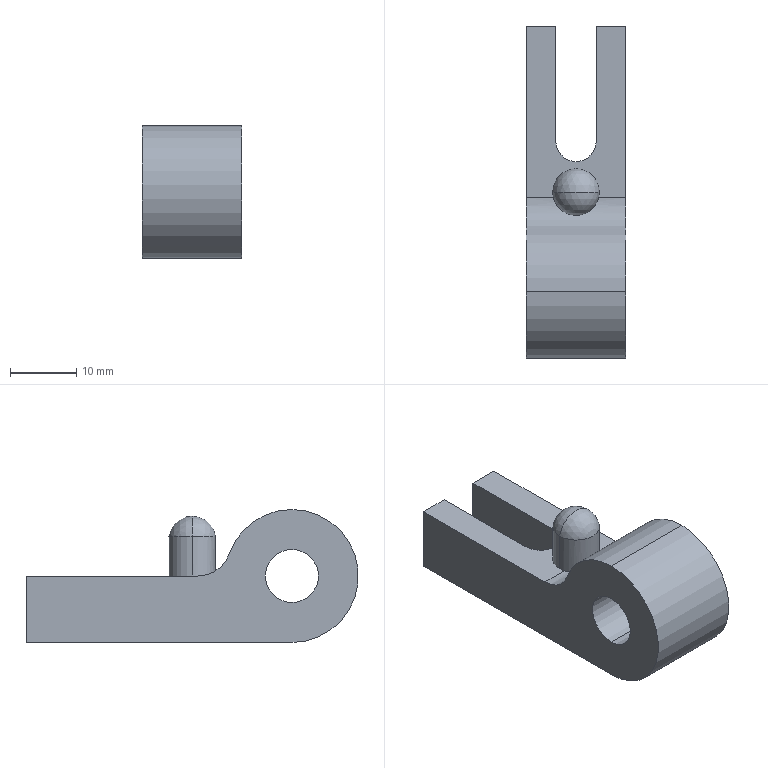Part | SolidWorks | features ICE 4, Fillet 2, Dome 1, Extrusion 1 | 1 solid | 18 faces | box 15 x 50 x 20 mm | volume 7920 mm3 | cylinder 8 | plane 8 | sphere 2 | commonest cylinder face diameters 7 x2 8 x2 20 x2 6.1 x1 10 x1
STEP:
#1=CARTESIAN_POINT('',(3.5,25.,6.));
#2=VERTEX_POINT('',#1);
#3=CARTESIAN_POINT('',(-3.5,25.,6.));
#4=VERTEX_POINT('',#3);
#5=CARTESIAN_POINT('',(0.,25.,6.));
#6=DIRECTION('',(0.,0.,1.));
#7=DIRECTION('',(1.,0.,0.));
#8=AXIS2_PLACEMENT_3D('',#5,#6,#7);
#9=CIRCLE('',#8,3.5);
#10=EDGE_CURVE('',#2,#4,#9,.T.);
#11=ORIENTED_EDGE('',*,*,#10,.T.);
#12=CARTESIAN_POINT('',(0.,25.,9.));
#13=VERTEX_POINT('',#12);
#14=CARTESIAN_POINT('',(0.,25.,5.458));
#15=DIRECTION('',(0.,1.,0.));
#16=DIRECTION('',(-1.,0.,0.));
#17=AXIS2_PLACEMENT_3D('',#14,#15,#16);
#18=CIRCLE('',#17,3.542);
#19=EDGE_CURVE('',#4,#13,#18,.T.);
#20=ORIENTED_EDGE('',*,*,#19,.T.);
#21=CARTESIAN_POINT('',(0.,25.,5.458));
#22=DIRECTION('',(0.,-1.,0.));
#23=DIRECTION('',(0.,0.,-1.));
#24=AXIS2_PLACEMENT_3D('',#21,#22,#23);
#25=CIRCLE('',#24,3.542);
#26=EDGE_CURVE('',#2,#13,#25,.T.);
#27=ORIENTED_EDGE('',*,*,#26,.F.);
#28=EDGE_LOOP('',(#11,#20,#27));
#29=FACE_OUTER_BOUND('',#28,.T.);
#30=CARTESIAN_POINT('',(0.,25.,5.458));
#31=DIRECTION('',(0.,1.,0.));
#32=DIRECTION('',(1.,0.,0.));
#33=AXIS2_PLACEMENT_3D('',#30,#31,#32);
#34=SPHERICAL_SURFACE('',#33,3.542);
#35=ADVANCED_FACE('',(#29),#34,.T.);
#36=ORIENTED_EDGE('',*,*,#10,.F.);
#37=CARTESIAN_POINT('',(3.5,25.,0.));
#38=VERTEX_POINT('',#37);
#39=CARTESIAN_POINT('',(3.5,25.,6.));
#40=DIRECTION('',(0.,0.,-1.));
#41=VECTOR('',#40,1000.);
#42=LINE('',#39,#41);
#43=EDGE_CURVE('',#2,#38,#42,.T.);
#44=ORIENTED_EDGE('',*,*,#43,.T.);
#45=CARTESIAN_POINT('',(-3.5,25.,0.));
#46=VERTEX_POINT('',#45);
#47=CARTESIAN_POINT('',(0.,25.,0.));
#48=DIRECTION('',(0.,0.,1.));
#49=DIRECTION('',(1.,0.,0.));
#50=AXIS2_PLACEMENT_3D('',#47,#48,#49);
#51=CIRCLE('',#50,3.5);
#52=EDGE_CURVE('',#38,#46,#51,.T.);
#53=ORIENTED_EDGE('',*,*,#52,.T.);
#54=CARTESIAN_POINT('',(-3.5,25.,6.));
#55=DIRECTION('',(0.,0.,-1.));
#56=VECTOR('',#55,1000.);
#57=LINE('',#54,#56);
#58=EDGE_CURVE('',#4,#46,#57,.T.);
#59=ORIENTED_EDGE('',*,*,#58,.F.);
#60=EDGE_LOOP('',(#36,#44,#53,#59));
#61=FACE_OUTER_BOUND('',#60,.T.);
#62=CARTESIAN_POINT('',(0.,25.,6.));
#63=DIRECTION('',(0.,0.,-1.));
#64=DIRECTION('',(-1.,0.,0.));
#65=AXIS2_PLACEMENT_3D('',#62,#63,#64);
#66=CYLINDRICAL_SURFACE('',#65,3.5);
#67=ADVANCED_FACE('',(#61),#66,.T.);
#68=CARTESIAN_POINT('',(7.5,10.,-4.));
#69=VERTEX_POINT('',#68);
#70=CARTESIAN_POINT('',(7.5,10.,4.));
#71=VERTEX_POINT('',#70);
#72=CARTESIAN_POINT('',(7.5,10.,0.));
#73=DIRECTION('',(-1.,0.,0.));
#74=DIRECTION('',(0.,0.,1.));
#75=AXIS2_PLACEMENT_3D('',#72,#73,#74);
#76=CIRCLE('',#75,4.);
#77=EDGE_CURVE('',#69,#71,#76,.T.);
#78=ORIENTED_EDGE('',*,*,#77,.F.);
#79=CARTESIAN_POINT('',(-7.5,10.,-4.));
#80=VERTEX_POINT('',#79);
#81=CARTESIAN_POINT('',(7.5,10.,-4.));
#82=DIRECTION('',(-1.,0.,0.));
#83=VECTOR('',#82,1000.);
#84=LINE('',#81,#83);
#85=EDGE_CURVE('',#69,#80,#84,.T.);
#86=ORIENTED_EDGE('',*,*,#85,.T.);
#87=CARTESIAN_POINT('',(-7.5,10.,4.));
#88=VERTEX_POINT('',#87);
#89=CARTESIAN_POINT('',(-7.5,10.,0.));
#90=DIRECTION('',(-1.,0.,0.));
#91=DIRECTION('',(0.,0.,1.));
#92=AXIS2_PLACEMENT_3D('',#89,#90,#91);
#93=CIRCLE('',#92,4.);
#94=EDGE_CURVE('',#80,#88,#93,.T.);
#95=ORIENTED_EDGE('',*,*,#94,.T.);
#96=CARTESIAN_POINT('',(7.5,10.,4.));
#97=DIRECTION('',(-1.,0.,0.));
#98=VECTOR('',#97,1000.);
#99=LINE('',#96,#98);
#100=EDGE_CURVE('',#71,#88,#99,.T.);
#101=ORIENTED_EDGE('',*,*,#100,.F.);
#102=EDGE_LOOP('',(#78,#86,#95,#101));
#103=FACE_OUTER_BOUND('',#102,.T.);
#104=CARTESIAN_POINT('',(7.5,10.,0.));
#105=DIRECTION('',(-1.,0.,0.));
#106=DIRECTION('',(0.,0.,1.));
#107=AXIS2_PLACEMENT_3D('',#104,#105,#106);
#108=CYLINDRICAL_SURFACE('',#107,4.);
#109=ADVANCED_FACE('',(#103),#108,.F.);
#110=CARTESIAN_POINT('',(7.5,10.,10.));
#111=VERTEX_POINT('',#110);
#112=CARTESIAN_POINT('',(7.5,10.,-10.));
#113=VERTEX_POINT('',#112);
#114=CARTESIAN_POINT('',(7.5,10.,0.));
#115=DIRECTION('',(1.,0.,0.));
#116=DIRECTION('',(0.,0.,1.));
#117=AXIS2_PLACEMENT_3D('',#114,#115,#116);
#118=CIRCLE('',#117,10.);
#119=EDGE_CURVE('',#111,#113,#118,.T.);
#120=ORIENTED_EDGE('',*,*,#119,.F.);
#121=CARTESIAN_POINT('',(-7.5,10.,10.));
#122=VERTEX_POINT('',#121);
#123=CARTESIAN_POINT('',(7.5,10.,10.));
#124=DIRECTION('',(-1.,0.,0.));
#125=VECTOR('',#124,1000.);
#126=LINE('',#123,#125);
#127=EDGE_CURVE('',#111,#122,#126,.T.);
#128=ORIENTED_EDGE('',*,*,#127,.T.);
#129=CARTESIAN_POINT('',(-7.5,10.,-10.));
#130=VERTEX_POINT('',#129);
#131=CARTESIAN_POINT('',(-7.5,10.,0.));
#132=DIRECTION('',(-1.,0.,0.));
#133=DIRECTION('',(0.,0.,-1.));
#134=AXIS2_PLACEMENT_3D('',#131,#132,#133);
#135=CIRCLE('',#134,10.);
#136=EDGE_CURVE('',#130,#122,#135,.T.);
#137=ORIENTED_EDGE('',*,*,#136,.F.);
#138=CARTESIAN_POINT('',(7.5,10.,-10.));
#139=DIRECTION('',(-1.,0.,0.));
#140=VECTOR('',#139,1000.);
#141=LINE('',#138,#140);
#142=EDGE_CURVE('',#113,#130,#141,.T.);
#143=ORIENTED_EDGE('',*,*,#142,.F.);
#144=EDGE_LOOP('',(#120,#128,#137,#143));
#145=FACE_OUTER_BOUND('',#144,.T.);
#146=CARTESIAN_POINT('',(7.5,10.,0.));
#147=DIRECTION('',(-1.,0.,0.));
#148=DIRECTION('',(0.,0.,1.));
#149=AXIS2_PLACEMENT_3D('',#146,#147,#148);
#150=CYLINDRICAL_SURFACE('',#149,10.);
#151=ADVANCED_FACE('',(#145),#150,.T.);
#152=CARTESIAN_POINT('',(-3.05,50.,0.));
#153=VERTEX_POINT('',#152);
#154=CARTESIAN_POINT('',(-7.5,50.,0.));
#155=VERTEX_POINT('',#154);
#156=CARTESIAN_POINT('',(7.5,50.,0.));
#157=DIRECTION('',(-1.,0.,0.));
#158=VECTOR('',#157,1000.);
#159=LINE('',#156,#158);
#160=EDGE_CURVE('',#153,#155,#159,.T.);
#161=ORIENTED_EDGE('',*,*,#160,.F.);
#162=CARTESIAN_POINT('',(-3.05,50.,-10.));
#163=VERTEX_POINT('',#162);
#164=CARTESIAN_POINT('',(-3.05,50.,10.));
#165=DIRECTION('',(0.,0.,-1.));
#166=VECTOR('',#165,1000.);
#167=LINE('',#164,#166);
#168=EDGE_CURVE('',#153,#163,#167,.T.);
#169=ORIENTED_EDGE('',*,*,#168,.T.);
#170=CARTESIAN_POINT('',(-7.5,50.,-10.));
#171=VERTEX_POINT('',#170);
#172=CARTESIAN_POINT('',(-7.5,50.,-10.));
#173=DIRECTION('',(-1.,0.,0.));
#174=VECTOR('',#173,1000.);
#175=LINE('',#172,#174);
#176=EDGE_CURVE('',#163,#171,#175,.T.);
#177=ORIENTED_EDGE('',*,*,#176,.T.);
#178=CARTESIAN_POINT('',(-7.5,50.,10.));
#179=DIRECTION('',(0.,0.,1.));
#180=VECTOR('',#179,1000.);
#181=LINE('',#178,#180);
#182=EDGE_CURVE('',#171,#155,#181,.T.);
#183=ORIENTED_EDGE('',*,*,#182,.T.);
#184=EDGE_LOOP('',(#161,#169,#177,#183));
#185=FACE_OUTER_BOUND('',#184,.T.);
#186=CARTESIAN_POINT('',(0.,50.,0.));
#187=DIRECTION('',(0.,-1.,0.));
#188=DIRECTION('',(0.,0.,-1.));
#189=AXIS2_PLACEMENT_3D('',#186,#187,#188);
#190=PLANE('',#189);
#191=ADVANCED_FACE('',(#185),#190,.F.);
#192=CARTESIAN_POINT('',(-3.393,24.142,0.));
#193=VERTEX_POINT('',#192);
#194=CARTESIAN_POINT('',(3.393,24.142,0.));
#195=VERTEX_POINT('',#194);
#196=CARTESIAN_POINT('',(-3.393,24.142,0.));
#197=CARTESIAN_POINT('',(-3.345,23.95,0.));
#198=CARTESIAN_POINT('',(-3.281,23.766,0.011));
#199=CARTESIAN_POINT('',(-3.124,23.411,0.05057));
#200=CARTESIAN_POINT('',(-3.031,23.239,0.0794));
#201=CARTESIAN_POINT('',(-2.818,22.915,0.1501));
#202=CARTESIAN_POINT('',(-2.7,22.765,0.1913));
#203=CARTESIAN_POINT('',(-2.441,22.485,0.2804));
#204=CARTESIAN_POINT('',(-2.3,22.355,0.3287));
#205=CARTESIAN_POINT('',(-1.999,22.121,0.4251));
#206=CARTESIAN_POINT('',(-1.841,22.017,0.4729));
#207=CARTESIAN_POINT('',(-1.507,21.835,0.5628));
#208=CARTESIAN_POINT('',(-1.33,21.757,0.6051));
#209=CARTESIAN_POINT('',(-0.9648,21.63,0.6763));
#210=CARTESIAN_POINT('',(-0.7783,21.582,0.7049));
#211=CARTESIAN_POINT('',(-0.3972,21.517,0.7443));
#212=CARTESIAN_POINT('',(-0.2008,21.5,0.755));
#213=CARTESIAN_POINT('',(0.1939,21.5,0.7552));
#214=CARTESIAN_POINT('',(0.3883,21.516,0.7449));
#215=CARTESIAN_POINT('',(0.7717,21.581,0.7058));
#216=CARTESIAN_POINT('',(0.9624,21.629,0.6767));
#217=CARTESIAN_POINT('',(1.328,21.756,0.6055));
#218=CARTESIAN_POINT('',(1.503,21.833,0.5638));
#219=CARTESIAN_POINT('',(1.839,22.016,0.4735));
#220=CARTESIAN_POINT('',(2.,22.121,0.4247));
#221=CARTESIAN_POINT('',(2.3,22.355,0.3287));
#222=CARTESIAN_POINT('',(2.439,22.483,0.2811));
#223=CARTESIAN_POINT('',(2.699,22.763,0.1916));
#224=CARTESIAN_POINT('',(2.819,22.917,0.1497));
#225=CARTESIAN_POINT('',(3.03,23.238,0.07977));
#226=CARTESIAN_POINT('',(3.122,23.406,0.05121));
#227=CARTESIAN_POINT('',(3.279,23.762,0.01128));
#228=CARTESIAN_POINT('',(3.345,23.95,0.));
#229=CARTESIAN_POINT('',(3.393,24.142,0.));
#230=B_SPLINE_CURVE_WITH_KNOTS('',3,(#196,#197,#198,#199,#200,#201,#202,#203,#204,#205,#206,#207,#208,#209,#210,#211,#212,#213,#214,#215,#216,#217,#218,#219,#220,#221,#222,#223,#224,#225,#226,#227,#228,#229),.UNSPECIFIED.,.F.,.F.,(4,2,2,2,2,2,2,2,2,2,2,2,2,2,2,2,4),(0.,0.0005847,0.001169,0.001754,0.002339,0.002924,0.003508,0.004093,0.004678,0.005262,0.005847,0.006432,0.007017,0.007601,0.008186,0.008771,0.009355),.UNSPECIFIED.);
#231=EDGE_CURVE('',#193,#195,#230,.T.);
#232=ORIENTED_EDGE('',*,*,#231,.F.);
#233=CARTESIAN_POINT('',(-7.5,24.142,0.));
#234=VERTEX_POINT('',#233);
#235=CARTESIAN_POINT('',(7.5,24.142,0.));
#236=DIRECTION('',(1.,0.,0.));
#237=VECTOR('',#236,1000.);
#238=LINE('',#235,#237);
#239=EDGE_CURVE('',#234,#193,#238,.T.);
#240=ORIENTED_EDGE('',*,*,#239,.F.);
#241=CARTESIAN_POINT('',(-7.5,19.428,3.333));
#242=VERTEX_POINT('',#241);
#243=CARTESIAN_POINT('',(-7.5,24.142,5.));
#244=DIRECTION('',(1.,0.,0.));
#245=DIRECTION('',(0.,0.,-1.));
#246=AXIS2_PLACEMENT_3D('',#243,#244,#245);
#247=CIRCLE('',#246,5.);
#248=EDGE_CURVE('',#242,#234,#247,.T.);
#249=ORIENTED_EDGE('',*,*,#248,.F.);
#250=CARTESIAN_POINT('',(7.5,19.428,3.333));
#251=VERTEX_POINT('',#250);
#252=CARTESIAN_POINT('',(7.5,19.428,3.333));
#253=DIRECTION('',(-1.,0.,0.));
#254=VECTOR('',#253,1000.);
#255=LINE('',#252,#254);
#256=EDGE_CURVE('',#251,#242,#255,.T.);
#257=ORIENTED_EDGE('',*,*,#256,.F.);
#258=CARTESIAN_POINT('',(7.5,24.142,0.));
#259=VERTEX_POINT('',#258);
#260=CARTESIAN_POINT('',(7.5,24.142,5.));
#261=DIRECTION('',(-1.,0.,0.));
#262=DIRECTION('',(0.,0.,1.));
#263=AXIS2_PLACEMENT_3D('',#260,#261,#262);
#264=CIRCLE('',#263,5.);
#265=EDGE_CURVE('',#259,#251,#264,.T.);
#266=ORIENTED_EDGE('',*,*,#265,.F.);
#267=CARTESIAN_POINT('',(7.5,24.142,0.));
#268=DIRECTION('',(1.,0.,0.));
#269=VECTOR('',#268,1000.);
#270=LINE('',#267,#269);
#271=EDGE_CURVE('',#195,#259,#270,.T.);
#272=ORIENTED_EDGE('',*,*,#271,.F.);
#273=EDGE_LOOP('',(#232,#240,#249,#257,#266,#272));
#274=FACE_OUTER_BOUND('',#273,.T.);
#275=CARTESIAN_POINT('',(7.5,24.142,5.));
#276=DIRECTION('',(-1.,0.,0.));
#277=DIRECTION('',(0.,0.,1.));
#278=AXIS2_PLACEMENT_3D('',#275,#276,#277);
#279=CYLINDRICAL_SURFACE('',#278,5.);
#280=ADVANCED_FACE('',(#274),#279,.F.);
#281=ORIENTED_EDGE('',*,*,#127,.F.);
#282=CARTESIAN_POINT('',(7.5,10.,0.));
#283=DIRECTION('',(1.,0.,0.));
#284=DIRECTION('',(0.,0.,1.));
#285=AXIS2_PLACEMENT_3D('',#282,#283,#284);
#286=CIRCLE('',#285,10.);
#287=EDGE_CURVE('',#251,#111,#286,.T.);
#288=ORIENTED_EDGE('',*,*,#287,.F.);
#289=ORIENTED_EDGE('',*,*,#256,.T.);
#290=CARTESIAN_POINT('',(-7.5,10.,0.));
#291=DIRECTION('',(-1.,0.,0.));
#292=DIRECTION('',(0.,0.,-1.));
#293=AXIS2_PLACEMENT_3D('',#290,#291,#292);
#294=CIRCLE('',#293,10.);
#295=EDGE_CURVE('',#122,#242,#294,.T.);
#296=ORIENTED_EDGE('',*,*,#295,.F.);
#297=EDGE_LOOP('',(#281,#288,#289,#296));
#298=FACE_OUTER_BOUND('',#297,.T.);
#299=CARTESIAN_POINT('',(7.5,10.,0.));
#300=DIRECTION('',(-1.,0.,0.));
#301=DIRECTION('',(0.,0.,1.));
#302=AXIS2_PLACEMENT_3D('',#299,#300,#301);
#303=CYLINDRICAL_SURFACE('',#302,10.);
#304=ADVANCED_FACE('',(#298),#303,.T.);
#305=CARTESIAN_POINT('',(7.5,10.,0.));
#306=DIRECTION('',(-1.,0.,0.));
#307=DIRECTION('',(0.,0.,1.));
#308=AXIS2_PLACEMENT_3D('',#305,#306,#307);
#309=CIRCLE('',#308,4.);
#310=EDGE_CURVE('',#71,#69,#309,.T.);
#311=ORIENTED_EDGE('',*,*,#310,.T.);
#312=ORIENTED_EDGE('',*,*,#77,.T.);
#313=EDGE_LOOP('',(#311,#312));
#314=FACE_BOUND('',#313,.T.);
#315=CARTESIAN_POINT('',(7.5,50.,0.));
#316=VERTEX_POINT('',#315);
#317=CARTESIAN_POINT('',(7.5,20.,0.));
#318=DIRECTION('',(0.,-1.,0.));
#319=VECTOR('',#318,1000.);
#320=LINE('',#317,#319);
#321=EDGE_CURVE('',#316,#259,#320,.T.);
#322=ORIENTED_EDGE('',*,*,#321,.T.);
#323=ORIENTED_EDGE('',*,*,#265,.T.);
#324=ORIENTED_EDGE('',*,*,#287,.T.);
#325=ORIENTED_EDGE('',*,*,#119,.T.);
#326=CARTESIAN_POINT('',(7.5,50.,-10.));
#327=VERTEX_POINT('',#326);
#328=CARTESIAN_POINT('',(7.5,50.,-10.));
#329=DIRECTION('',(0.,-1.,0.));
#330=VECTOR('',#329,1000.);
#331=LINE('',#328,#330);
#332=EDGE_CURVE('',#327,#113,#331,.T.);
#333=ORIENTED_EDGE('',*,*,#332,.F.);
#334=CARTESIAN_POINT('',(7.5,50.,10.));
#335=DIRECTION('',(0.,0.,-1.));
#336=VECTOR('',#335,1000.);
#337=LINE('',#334,#336);
#338=EDGE_CURVE('',#316,#327,#337,.T.);
#339=ORIENTED_EDGE('',*,*,#338,.F.);
#340=EDGE_LOOP('',(#322,#323,#324,#325,#333,#339));
#341=FACE_OUTER_BOUND('',#340,.T.);
#342=CARTESIAN_POINT('',(7.5,50.,10.));
#343=DIRECTION('',(-1.,0.,0.));
#344=DIRECTION('',(0.,0.,1.));
#345=AXIS2_PLACEMENT_3D('',#342,#343,#344);
#346=PLANE('',#345);
#347=ADVANCED_FACE('',(#314,#341),#346,.F.);
#348=ORIENTED_EDGE('',*,*,#176,.F.);
#349=CARTESIAN_POINT('',(-3.05,32.635,-10.));
#350=VERTEX_POINT('',#349);
#351=CARTESIAN_POINT('',(-3.05,50.,-10.));
#352=DIRECTION('',(0.,1.,0.));
#353=VECTOR('',#352,1000.);
#354=LINE('',#351,#353);
#355=EDGE_CURVE('',#350,#163,#354,.T.);
#356=ORIENTED_EDGE('',*,*,#355,.F.);
#357=CARTESIAN_POINT('',(3.05,32.635,-10.));
#358=VERTEX_POINT('',#357);
#359=CARTESIAN_POINT('',(0.,32.635,-10.));
#360=DIRECTION('',(0.,0.,-1.));
#361=DIRECTION('',(-1.,0.,0.));
#362=AXIS2_PLACEMENT_3D('',#359,#360,#361);
#363=CIRCLE('',#362,3.05);
#364=EDGE_CURVE('',#358,#350,#363,.T.);
#365=ORIENTED_EDGE('',*,*,#364,.F.);
#366=CARTESIAN_POINT('',(3.05,50.,-10.));
#367=VERTEX_POINT('',#366);
#368=CARTESIAN_POINT('',(3.05,50.,-10.));
#369=DIRECTION('',(0.,-1.,0.));
#370=VECTOR('',#369,1000.);
#371=LINE('',#368,#370);
#372=EDGE_CURVE('',#367,#358,#371,.T.);
#373=ORIENTED_EDGE('',*,*,#372,.F.);
#374=CARTESIAN_POINT('',(-7.5,50.,-10.));
#375=DIRECTION('',(-1.,0.,0.));
#376=VECTOR('',#375,1000.);
#377=LINE('',#374,#376);
#378=EDGE_CURVE('',#327,#367,#377,.T.);
#379=ORIENTED_EDGE('',*,*,#378,.F.);
#380=ORIENTED_EDGE('',*,*,#332,.T.);
#381=ORIENTED_EDGE('',*,*,#142,.T.);
#382=CARTESIAN_POINT('',(-7.5,50.,-10.));
#383=DIRECTION('',(0.,-1.,0.));
#384=VECTOR('',#383,1000.);
#385=LINE('',#382,#384);
#386=EDGE_CURVE('',#171,#130,#385,.T.);
#387=ORIENTED_EDGE('',*,*,#386,.F.);
#388=EDGE_LOOP('',(#348,#356,#365,#373,#379,#380,#381,#387));
#389=FACE_OUTER_BOUND('',#388,.T.);
#390=CARTESIAN_POINT('',(-7.5,50.,-10.));
#391=DIRECTION('',(0.,0.,1.));
#392=DIRECTION('',(1.,0.,0.));
#393=AXIS2_PLACEMENT_3D('',#390,#391,#392);
#394=PLANE('',#393);
#395=ADVANCED_FACE('',(#389),#394,.F.);
#396=CARTESIAN_POINT('',(-7.5,10.,0.));
#397=DIRECTION('',(-1.,0.,0.));
#398=DIRECTION('',(0.,0.,1.));
#399=AXIS2_PLACEMENT_3D('',#396,#397,#398);
#400=CIRCLE('',#399,4.);
#401=EDGE_CURVE('',#88,#80,#400,.T.);
#402=ORIENTED_EDGE('',*,*,#401,.F.);
#403=ORIENTED_EDGE('',*,*,#94,.F.);
#404=EDGE_LOOP('',(#402,#403));
#405=FACE_BOUND('',#404,.T.);
#406=ORIENTED_EDGE('',*,*,#136,.T.);
#407=ORIENTED_EDGE('',*,*,#295,.T.);
#408=ORIENTED_EDGE('',*,*,#248,.T.);
#409=CARTESIAN_POINT('',(-7.5,20.,0.));
#410=DIRECTION('',(0.,-1.,0.));
#411=VECTOR('',#410,1000.);
#412=LINE('',#409,#411);
#413=EDGE_CURVE('',#155,#234,#412,.T.);
#414=ORIENTED_EDGE('',*,*,#413,.F.);
#415=ORIENTED_EDGE('',*,*,#182,.F.);
#416=ORIENTED_EDGE('',*,*,#386,.T.);
#417=EDGE_LOOP('',(#406,#407,#408,#414,#415,#416));
#418=FACE_OUTER_BOUND('',#417,.T.);
#419=CARTESIAN_POINT('',(-7.5,50.,10.));
#420=DIRECTION('',(1.,0.,0.));
#421=DIRECTION('',(0.,0.,-1.));
#422=AXIS2_PLACEMENT_3D('',#419,#420,#421);
#423=PLANE('',#422);
#424=ADVANCED_FACE('',(#405,#418),#423,.F.);
#425=ORIENTED_EDGE('',*,*,#378,.T.);
#426=CARTESIAN_POINT('',(3.05,50.,0.));
#427=VERTEX_POINT('',#426);
#428=CARTESIAN_POINT('',(3.05,50.,10.));
#429=DIRECTION('',(0.,0.,-1.));
#430=VECTOR('',#429,1000.);
#431=LINE('',#428,#430);
#432=EDGE_CURVE('',#427,#367,#431,.T.);
#433=ORIENTED_EDGE('',*,*,#432,.F.);
#434=CARTESIAN_POINT('',(7.5,50.,0.));
#435=DIRECTION('',(-1.,0.,0.));
#436=VECTOR('',#435,1000.);
#437=LINE('',#434,#436);
#438=EDGE_CURVE('',#316,#427,#437,.T.);
#439=ORIENTED_EDGE('',*,*,#438,.F.);
#440=ORIENTED_EDGE('',*,*,#338,.T.);
#441=EDGE_LOOP('',(#425,#433,#439,#440));
#442=FACE_OUTER_BOUND('',#441,.T.);
#443=CARTESIAN_POINT('',(0.,50.,0.));
#444=DIRECTION('',(0.,-1.,0.));
#445=DIRECTION('',(0.,0.,-1.));
#446=AXIS2_PLACEMENT_3D('',#443,#444,#445);
#447=PLANE('',#446);
#448=ADVANCED_FACE('',(#442),#447,.F.);
#449=ORIENTED_EDGE('',*,*,#85,.F.);
#450=ORIENTED_EDGE('',*,*,#310,.F.);
#451=ORIENTED_EDGE('',*,*,#100,.T.);
#452=ORIENTED_EDGE('',*,*,#401,.T.);
#453=EDGE_LOOP('',(#449,#450,#451,#452));
#454=FACE_OUTER_BOUND('',#453,.T.);
#455=CARTESIAN_POINT('',(7.5,10.,0.));
#456=DIRECTION('',(-1.,0.,0.));
#457=DIRECTION('',(0.,0.,1.));
#458=AXIS2_PLACEMENT_3D('',#455,#456,#457);
#459=CYLINDRICAL_SURFACE('',#458,4.);
#460=ADVANCED_FACE('',(#454),#459,.F.);
#461=CARTESIAN_POINT('',(3.05,32.635,0.));
#462=VERTEX_POINT('',#461);
#463=CARTESIAN_POINT('',(-3.05,32.635,0.));
#464=VERTEX_POINT('',#463);
#465=CARTESIAN_POINT('',(0.,32.635,0.));
#466=DIRECTION('',(0.,0.,-1.));
#467=DIRECTION('',(-1.,0.,0.));
#468=AXIS2_PLACEMENT_3D('',#465,#466,#467);
#469=CIRCLE('',#468,3.05);
#470=EDGE_CURVE('',#462,#464,#469,.T.);
#471=ORIENTED_EDGE('',*,*,#470,.T.);
#472=CARTESIAN_POINT('',(-3.05,20.,0.));
#473=DIRECTION('',(0.,1.,0.));
#474=VECTOR('',#473,1000.);
#475=LINE('',#472,#474);
#476=EDGE_CURVE('',#464,#153,#475,.T.);
#477=ORIENTED_EDGE('',*,*,#476,.T.);
#478=ORIENTED_EDGE('',*,*,#160,.T.);
#479=ORIENTED_EDGE('',*,*,#413,.T.);
#480=ORIENTED_EDGE('',*,*,#239,.T.);
#481=CARTESIAN_POINT('',(0.,25.,0.));
#482=DIRECTION('',(0.,0.,1.));
#483=DIRECTION('',(1.,0.,0.));
#484=AXIS2_PLACEMENT_3D('',#481,#482,#483);
#485=CIRCLE('',#484,3.5);
#486=EDGE_CURVE('',#46,#193,#485,.T.);
#487=ORIENTED_EDGE('',*,*,#486,.F.);
#488=ORIENTED_EDGE('',*,*,#52,.F.);
#489=CARTESIAN_POINT('',(0.,25.,0.));
#490=DIRECTION('',(0.,0.,1.));
#491=DIRECTION('',(1.,0.,0.));
#492=AXIS2_PLACEMENT_3D('',#489,#490,#491);
#493=CIRCLE('',#492,3.5);
#494=EDGE_CURVE('',#195,#38,#493,.T.);
#495=ORIENTED_EDGE('',*,*,#494,.F.);
#496=ORIENTED_EDGE('',*,*,#271,.T.);
#497=ORIENTED_EDGE('',*,*,#321,.F.);
#498=ORIENTED_EDGE('',*,*,#438,.T.);
#499=CARTESIAN_POINT('',(3.05,20.,0.));
#500=DIRECTION('',(0.,-1.,0.));
#501=VECTOR('',#500,1000.);
#502=LINE('',#499,#501);
#503=EDGE_CURVE('',#427,#462,#502,.T.);
#504=ORIENTED_EDGE('',*,*,#503,.T.);
#505=EDGE_LOOP('',(#471,#477,#478,#479,#480,#487,#488,#495,#496,#497,#498,#504));
#506=FACE_OUTER_BOUND('',#505,.T.);
#507=CARTESIAN_POINT('',(7.5,20.,0.));
#508=DIRECTION('',(0.,0.,-1.));
#509=DIRECTION('',(-1.,0.,0.));
#510=AXIS2_PLACEMENT_3D('',#507,#508,#509);
#511=PLANE('',#510);
#512=ADVANCED_FACE('',(#506),#511,.F.);
#513=ORIENTED_EDGE('',*,*,#43,.F.);
#514=CARTESIAN_POINT('',(0.,25.,6.));
#515=DIRECTION('',(0.,0.,1.));
#516=DIRECTION('',(1.,0.,0.));
#517=AXIS2_PLACEMENT_3D('',#514,#515,#516);
#518=CIRCLE('',#517,3.5);
#519=EDGE_CURVE('',#4,#2,#518,.T.);
#520=ORIENTED_EDGE('',*,*,#519,.F.);
#521=ORIENTED_EDGE('',*,*,#58,.T.);
#522=ORIENTED_EDGE('',*,*,#486,.T.);
#523=ORIENTED_EDGE('',*,*,#231,.T.);
#524=ORIENTED_EDGE('',*,*,#494,.T.);
#525=EDGE_LOOP('',(#513,#520,#521,#522,#523,#524));
#526=FACE_OUTER_BOUND('',#525,.T.);
#527=CARTESIAN_POINT('',(0.,25.,6.));
#528=DIRECTION('',(0.,0.,-1.));
#529=DIRECTION('',(-1.,0.,0.));
#530=AXIS2_PLACEMENT_3D('',#527,#528,#529);
#531=CYLINDRICAL_SURFACE('',#530,3.5);
#532=ADVANCED_FACE('',(#526),#531,.T.);
#533=ORIENTED_EDGE('',*,*,#19,.F.);
#534=ORIENTED_EDGE('',*,*,#519,.T.);
#535=ORIENTED_EDGE('',*,*,#26,.T.);
#536=EDGE_LOOP('',(#533,#534,#535));
#537=FACE_OUTER_BOUND('',#536,.T.);
#538=CARTESIAN_POINT('',(0.,25.,5.458));
#539=DIRECTION('',(0.,1.,0.));
#540=DIRECTION('',(1.,0.,0.));
#541=AXIS2_PLACEMENT_3D('',#538,#539,#540);
#542=SPHERICAL_SURFACE('',#541,3.542);
#543=ADVANCED_FACE('',(#537),#542,.T.);
#544=CARTESIAN_POINT('',(-3.05,32.635,10.));
#545=DIRECTION('',(0.,0.,-1.));
#546=VECTOR('',#545,1000.);
#547=LINE('',#544,#546);
#548=EDGE_CURVE('',#464,#350,#547,.T.);
#549=ORIENTED_EDGE('',*,*,#548,.T.);
#550=ORIENTED_EDGE('',*,*,#355,.T.);
#551=ORIENTED_EDGE('',*,*,#168,.F.);
#552=ORIENTED_EDGE('',*,*,#476,.F.);
#553=EDGE_LOOP('',(#549,#550,#551,#552));
#554=FACE_OUTER_BOUND('',#553,.T.);
#555=CARTESIAN_POINT('',(-3.05,50.,10.));
#556=DIRECTION('',(-1.,0.,0.));
#557=DIRECTION('',(0.,-1.,0.));
#558=AXIS2_PLACEMENT_3D('',#555,#556,#557);
#559=PLANE('',#558);
#560=ADVANCED_FACE('',(#554),#559,.F.);
#561=CARTESIAN_POINT('',(3.05,32.635,10.));
#562=DIRECTION('',(0.,0.,-1.));
#563=VECTOR('',#562,1000.);
#564=LINE('',#561,#563);
#565=EDGE_CURVE('',#462,#358,#564,.T.);
#566=ORIENTED_EDGE('',*,*,#565,.T.);
#567=ORIENTED_EDGE('',*,*,#364,.T.);
#568=ORIENTED_EDGE('',*,*,#548,.F.);
#569=ORIENTED_EDGE('',*,*,#470,.F.);
#570=EDGE_LOOP('',(#566,#567,#568,#569));
#571=FACE_OUTER_BOUND('',#570,.T.);
#572=CARTESIAN_POINT('',(0.,32.635,10.));
#573=DIRECTION('',(0.,0.,-1.));
#574=DIRECTION('',(-1.,0.,0.));
#575=AXIS2_PLACEMENT_3D('',#572,#573,#574);
#576=CYLINDRICAL_SURFACE('',#575,3.05);
#577=ADVANCED_FACE('',(#571),#576,.F.);
#578=ORIENTED_EDGE('',*,*,#432,.T.);
#579=ORIENTED_EDGE('',*,*,#372,.T.);
#580=ORIENTED_EDGE('',*,*,#565,.F.);
#581=ORIENTED_EDGE('',*,*,#503,.F.);
#582=EDGE_LOOP('',(#578,#579,#580,#581));
#583=FACE_OUTER_BOUND('',#582,.T.);
#584=CARTESIAN_POINT('',(3.05,50.,10.));
#585=DIRECTION('',(1.,0.,0.));
#586=DIRECTION('',(0.,1.,0.));
#587=AXIS2_PLACEMENT_3D('',#584,#585,#586);
#588=PLANE('',#587);
#589=ADVANCED_FACE('',(#583),#588,.F.);
#590=CLOSED_SHELL('',(#35,#67,#109,#151,#191,#280,#304,#347,#395,#424,#448,#460,#512,#532,#543,#560,#577,#589));
#591=MANIFOLD_SOLID_BREP('',#590);
#592=CARTESIAN_POINT('',(0.,0.,0.));
#593=DIRECTION('',(0.,0.,1.));
#594=DIRECTION('',(1.,0.,0.));
#595=AXIS2_PLACEMENT_3D('',#592,#593,#594);
#596=(LENGTH_UNIT()NAMED_UNIT(*)SI_UNIT(.MILLI.,.METRE.));
#597=UNCERTAINTY_MEASURE_WITH_UNIT(LENGTH_MEASURE(0.00001),#596,'','');
#598=(NAMED_UNIT(*)PLANE_ANGLE_UNIT()SI_UNIT($,.RADIAN.));
#599=(NAMED_UNIT(*)SI_UNIT($,.STERADIAN.)SOLID_ANGLE_UNIT());
#600=(GEOMETRIC_REPRESENTATION_CONTEXT(3)GLOBAL_UNCERTAINTY_ASSIGNED_CONTEXT((#597))GLOBAL_UNIT_ASSIGNED_CONTEXT((#596,#598,#599))REPRESENTATION_CONTEXT('',''));
#601=ADVANCED_BREP_SHAPE_REPRESENTATION('',(#591,#595),#600);